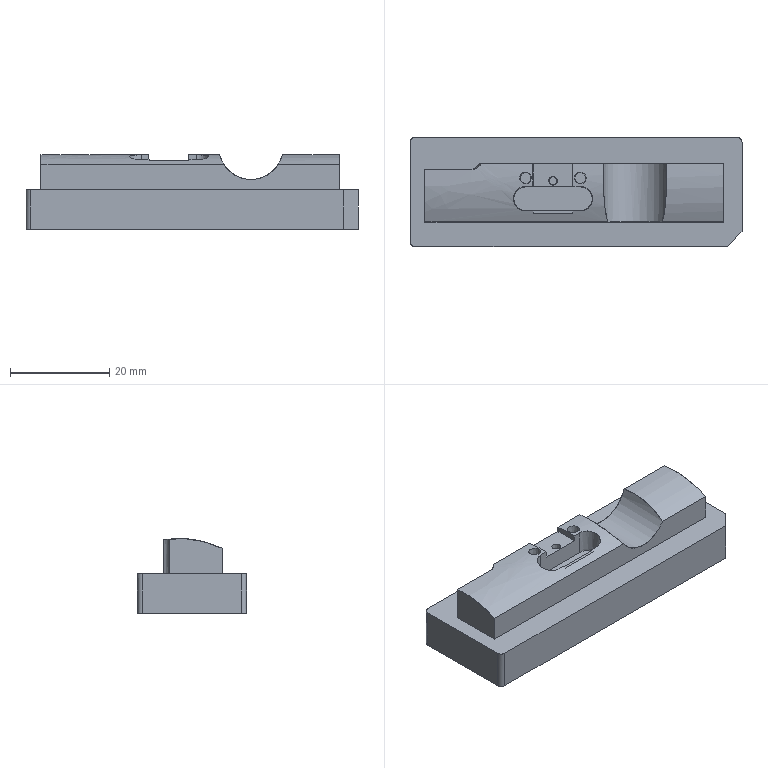NC program | PowerMill | posted with a generic post | part box 67 x 22 x 15.086 mm
Lines 3613 to 4616 of 221347:
N3710 M6
N3711 S18000 M03
N3712 G00 G90 X0.0 Y0.0
N3713 G43 Z9.7955 H15
N3714
N3715 G05 P10000 R4
N3716 X-0.6332 Y7.3349
N3717 Z0.8484
N3718 G01 Z-0.3516 F3000.0
N3719 Y7.1424 F5000.0
N3720 Y6.6108
N3721 X4.8545
N3722 X5.6988 Y6.6067
N3723 X6.1209 Y6.5128
N3724 X6.5431 Y6.2684
N3725 X6.6925 Y6.1209
N3726 X6.9624 Y5.6988
N3727 X7.0797 Y5.2767
N3728 X7.09 Y4.8545
N3729 X7.0958 Y1.0553
N3730 X7.0893 Y0.2111
N3731 X7.042 Y-0.2111
N3732 X6.9652 Y-0.4387
N3733 X6.8564 Y-0.6332
N3734 X6.4683 Y-1.0553
N3735 X6.1209 Y-1.2444
N3736 X5.6988 Y-1.3397
N3737 X2.7439 Y-1.3535
N3738 X2.3217 Y-1.2795
N3739 X1.8996 Y-1.0606
N3740 X1.4616 Y-0.6332
N3741 X1.2676 Y-0.5134
N3742 X1.0553 Y-0.4422
N3743 X1.0353 Y-0.4412
N3744 X0.6332 Y-0.42
N3745 X0.6293
N3746 X-0.6332
N3747 X-1.0553 Y-0.3626
N3748 X-1.4072 Y-0.2111
N3749 X-1.8666 Y0.2111
N3750 X-2.0765 Y0.6332
N3751 X-2.1447 Y1.0553
N3752 X-2.1446 Y4.8545
N3753 X-2.1353 Y5.2767
N3754 X-2.0179 Y5.6988
N3755 X-1.8996 Y5.9318
N3756 X-1.741 Y6.1209
N3757 X-1.4775 Y6.357
N3758 X-1.0553 Y6.5522
N3759 X-0.6332 Y6.6108
N3760 Y7.1424
N3761 G00 Z3.8484
N3762 G01 X-8.5382 Y7.3222 F10000.0
N3763 G00 Z0.8484
N3764 G01 Z-0.3516 F3000.0
N3765 X-8.569 Y7.1322 F5000.0
N3766 X-8.6537 Y6.6106
N3767 X-8.2316 Y6.542
N3768 X-7.8095 Y6.3319
N3769 X-7.5804 Y6.1209
N3770 X-7.3873 Y5.8707
N3771 X-7.3037 Y5.6988
N3772 X-7.1909 Y5.2767
N3773 X-7.1851 Y4.8545
N3774 X-7.1849 Y3.0772
N3775 X-5.3106
N3776 G02 X-4.1106 I0.6 J0.0
N3777 G02 X-5.3106 I-0.6 J0.0
N3778 G01 X-7.1849
N3779 X-7.1846 Y1.0553
N3780 X-7.2492 Y0.6332
N3781 X-7.3873 Y0.3236
N3782 X-7.4657 Y0.2111
N3783 X-7.8095 Y-0.1403
N3784 X-8.2316 Y-0.3475
N3785 X-8.6537 Y-0.4198
N3786 X-9.9201 Y-0.42
N3787 X-10.3423 Y-0.4421
N3788 X-10.557 Y-0.5125
N3789 X-10.7525 Y-0.6332
N3790 X-10.7642 Y-0.6446
N3791 X-10.7644 Y-0.6448
N3792 X-11.1848 Y-1.0553
N3793 X-11.6087 Y-1.2773
N3794 X-12.0308 Y-1.3551
N3795 X-19.6292 Y-1.3195
N3796 X-21.7399 Y-1.2703
N3797 X-29.7604 Y-1.2535
N3798 X-30.1825 Y-1.3112
N3799 X-30.6047 Y-1.3346
N3800 X-31.0268 Y-1.2356
N3801 X-31.4489 Y-0.9787
N3802 X-31.7472 Y-0.6332
N3803 X-31.8711 Y-0.3932
N3804 X-31.9294 Y-0.2111
N3805 X-31.9767 Y0.2111
N3806 Y4.4324
N3807 X-31.936 Y4.8545
N3808 X-31.8711 Y5.0606
N3809 X-31.7646 Y5.2767
N3810 X-31.4489 Y5.6498
N3811 X-31.0268 Y5.903
N3812 X-30.6047 Y6.002
N3813 X-30.1825 Y6.0075
N3814 X-21.1046 Y6.0103
N3815 X-20.8956 Y6.0394
N3816 X-20.7182 Y6.1209
N3817 X-20.4735 Y6.3206
N3818 X-20.0513 Y6.528
N3819 X-19.6292 Y6.6027
N3820 X-19.2071 Y6.6102
N3821 X-8.6537 Y6.6106
N3822 X-8.569 Y7.1322
N3823 G00 Z3.7118
N3824 G01 X6.2728 Y-2.9748 F10000.0
N3825 G00 Z0.7118
N3826 G01 Z-0.4882 F3000.0
N3827 X6.236 Y-2.7859 F5000.0
N3828 X6.1209 Y-2.1942
N3829 X5.6988 Y-2.2763
N3830 X3.166 Y-2.2705
N3831 X2.7439 Y-2.1871
N3832 X2.3217 Y-1.9541
N3833 X1.9254 Y-1.4775
N3834 X1.7658 Y-1.0553
N3835 X1.6513 Y-0.8317
N3836 X1.4881 Y-0.659
N3837 X1.4749 Y-0.6462
N3838 X1.2667 Y-0.5142
N3839 X1.0553 Y-0.4443
N3840 X0.6332 Y-0.4212
N3841 X0.6292
N3842 X-0.6332
N3843 X-1.0553 Y-0.3637
N3844 X-1.409 Y-0.2111
N3845 X-1.8675 Y0.2111
N3846 X-2.0765 Y0.6332
N3847 X-2.1447 Y1.0553
N3848 X-2.1446 Y2.2992
N3849 X-2.1445 Y4.8545
N3850 X-2.1444 Y4.8604
N3851 X-2.1443 Y5.6988
N3852 X-2.0862 Y6.1209
N3853 X-1.8996 Y6.5287
N3854 X-1.4775 Y6.9549
N3855 X-1.0553 Y7.1501
N3856 X-0.6332 Y7.2075
N3857 X5.2767
N3858 X5.6988 Y7.201
N3859 X6.1209 Y7.1257
N3860 X6.5431 Y6.8983
N3861 X6.8779 Y6.5431
N3862 X6.9652 Y6.3946
N3863 X7.074 Y6.1209
N3864 X7.1321 Y5.6988
N3865 X7.1391 Y0.2111
N3866 X7.1306 Y-0.6332
N3867 X7.0994 Y-1.0553
N3868 X6.9652 Y-1.4541
N3869 X6.6217 Y-1.8996
N3870 X6.5431 Y-1.965
N3871 X6.1209 Y-2.1942
N3872 X6.236 Y-2.7859
N3873 G00 Z3.7118
N3874 G01 X-30.7864 Y-3.0115 F10000.0
N3875 G00 Z0.7118
N3876 G01 Z-0.4882 F3000.0
N3877 X-30.7424 Y-2.8241 F5000.0
N3878 X-30.6047 Y-2.2385
N3879 X-31.0268 Y-2.1392
N3880 X-31.4489 Y-1.8933
N3881 X-31.7811 Y-1.4775
N3882 X-31.8711 Y-1.2977
N3883 X-31.9434 Y-1.0553
N3884 X-31.9767 Y-0.6332
N3885 Y4.4324
N3886 X-31.936 Y4.8545
N3887 X-31.8711 Y5.0606
N3888 X-31.7646 Y5.2767
N3889 X-31.4489 Y5.6498
N3890 X-31.0268 Y5.903
N3891 X-30.6047 Y6.002
N3892 X-30.1825 Y6.0075
N3893 X-30.0141
N3894 X-21.283 Y6.0102
N3895 X-21.2773 Y6.0106
N3896 X-20.8956 Y6.0402
N3897 X-20.7218 Y6.1209
N3898 X-20.5788 Y6.2528
N3899 X-20.3973 Y6.5431
N3900 X-20.0513 Y6.9071
N3901 X-19.6292 Y7.1274
N3902 X-19.2071 Y7.1966
N3903 X-18.7849 Y7.2075
N3904 X-8.6537 Y7.2073
N3905 X-8.2316 Y7.1271
N3906 X-7.8661 Y6.9652
N3907 X-7.4343 Y6.5431
N3908 X-7.2398 Y6.1209
N3909 X-7.184 Y5.6988
N3910 X-7.1836 Y3.7039
N3911 X-5.3179 Y3.7135
N3912 G02 X-4.7181 Y4.3166 I0.6 J0.0031
N3913 G01 X-4.6106
N3914 G02 X-4.0104 Y3.7137 I0.0002 J-0.6
N3915 G01 X-4.0136 Y3.071
N3916 G02 X-4.6144 Y2.474 I-0.6 J0.003
N3917 G01 X-4.7154 Y2.4741
N3918 G02 X-5.3146 Y3.071 I0.0008 J0.6
N3919 G01 X-5.3179 Y3.7135
N3920 X-7.1836 Y3.7039
N3921 X-7.1831 Y1.0553
N3922 X-7.2481 Y0.6332
N3923 X-7.3873 Y0.3207
N3924 X-7.4618 Y0.2111
N3925 X-7.8095 Y-0.1422
N3926 X-8.2316 Y-0.3504
N3927 X-8.6537 Y-0.421
N3928 X-9.9201 Y-0.4212
N3929 X-10.3423 Y-0.444
N3930 X-10.5561 Y-0.5133
N3931 X-10.7507 Y-0.6332
N3932 X-10.9407 Y-0.8297
N3933 X-11.0061 Y-0.9419
N3934 X-11.1865 Y-1.4214
N3935 X-11.5545 Y-1.8996
N3936 X-12.0308 Y-2.1853
N3937 X-12.4529 Y-2.2745
N3938 X-21.5288 Y-2.248
N3939 X-30.6047 Y-2.2385
N3940 X-30.7424 Y-2.8241
N3941 G00 Z3.5751
N3942 G01 X6.2495 Y-3.701 F10000.0
N3943 G00 Z0.5751
N3944 G01 Z-0.6249 F3000.0
N3945 X6.2187 Y-3.511 F5000.0
N3946 X6.1209 Y-2.9087
N3947 X5.6988 Y-2.9772
N3948 X3.166 Y-2.9741
N3949 X2.7439 Y-2.8638
N3950 X2.5152 Y-2.7439
N3951 X2.3217 Y-2.5996
N3952 X2.0811 Y-2.3217
N3953 X1.8825 Y-1.8996
N3954 X1.8231 Y-1.3709
N3955 X1.7646 Y-1.0553
N3956 X1.6505 Y-0.8325
N3957 X1.4775 Y-0.6493
N3958 X1.2659 Y-0.5151
N3959 X1.0553 Y-0.4465
N3960 X1.0363 Y-0.4454
N3961 X0.6332 Y-0.4224
N3962 X-0.6332
N3963 X-1.0553 Y-0.3647
N3964 X-1.4108 Y-0.2111
N3965 X-1.8679 Y0.2111
N3966 X-2.0765 Y0.6332
N3967 X-2.1447 Y1.0553
N3968 X-2.1445 Y3.0729
N3969 X-4.012 Y3.0724
N3970 G02 X-4.6127 Y2.4723 I-0.6 J-0.0001
N3971 G01 X-4.7153 Y2.4724
N3972 G02 X-5.3146 Y3.0725 I0.0007 J0.6
N3973 G01 X-5.3145 Y3.7085
N3974 G02 X-4.715 Y4.3083 I0.6 J-0.0002
N3975 G01 X-4.6128 Y4.3084
N3976 G02 X-4.0122 Y3.7086 I0.0006 J-0.6
N3977 G01 X-4.012 Y3.0724
N3978 X-2.1445 Y3.0729
N3979 Y3.5561
N3980 Y4.8545
N3981 X-2.1444 Y4.8575
N3982 X-2.1443 Y5.6988
N3983 X-2.0863 Y6.1209
N3984 X-1.8996 Y6.5287
N3985 X-1.4775 Y6.9549
N3986 X-1.0553 Y7.1501
N3987 X-0.6332 Y7.2075
N3988 X5.6988 Y7.2074
N3989 X6.1209 Y7.1401
N3990 X6.4963 Y6.9652
N3991 X6.9245 Y6.5431
N3992 X7.1207 Y6.1209
N3993 X7.1787 Y5.6988
N3994 X7.175 Y2.7439
N3995 X7.1818 Y-0.2111
N3996 X7.1685 Y-1.4775
N3997 X7.1065 Y-1.8996
N3998 X6.9074 Y-2.3217
N3999 X6.4747 Y-2.7439
N4000 X6.1209 Y-2.9087
N4001 X6.2187 Y-3.511
N4002 G00 Z3.5751
N4003 G01 X-31.3963 Y-3.5933 F10000.0
N4004 G00 Z0.5751
N4005 G01 Z-0.6249 F3000.0
N4006 X-31.3081 Y-3.4222 F5000.0
N4007 X-31.0268 Y-2.8762
N4008 X-31.2837 Y-2.7439
N4009 X-31.4489 Y-2.6222
N4010 X-31.7156 Y-2.3217
N4011 X-31.8711 Y-2.0325
N4012 X-31.9169 Y-1.8996
N4013 X-31.9767 Y-1.4775
N4014 Y4.4324
N4015 X-31.936 Y4.8545
N4016 X-31.8711 Y5.0606
N4017 X-31.7646 Y5.2767
N4018 X-31.4489 Y5.6498
N4019 X-31.0268 Y5.903
N4020 X-30.6047 Y6.002
N4021 X-30.1825 Y6.0075
N4022 X-29.8456
N4023 X-21.2861 Y6.0101
N4024 X-21.28 Y6.0106
N4025 X-20.8956 Y6.0427
N4026 X-20.729 Y6.1209
N4027 X-20.6745 Y6.1645
N4028 X-20.6467 Y6.1901
N4029 X-20.4045 Y6.5431
N4030 X-20.0513 Y6.9127
N4031 X-19.6292 Y7.1302
N4032 X-19.2071 Y7.199
N4033 X-18.7849 Y7.2075
N4034 X-8.6537 Y7.2073
N4035 X-8.2316 Y7.1294
N4036 X-7.8649 Y6.9652
N4037 X-7.4338 Y6.5431
N4038 X-7.2385 Y6.1209
N4039 X-7.1824 Y5.6988
N4040 X-7.1816 Y1.0553
N4041 X-7.247 Y0.6332
N4042 X-7.3873 Y0.3177
N4043 X-7.4579 Y0.2111
N4044 X-7.8095 Y-0.144
N4045 X-8.2316 Y-0.3533
N4046 X-8.6537 Y-0.4222
N4047 X-9.9201 Y-0.4224
N4048 X-10.3423 Y-0.446
N4049 X-10.5552 Y-0.5142
N4050 X-10.7488 Y-0.6332
N4051 X-10.9398 Y-0.8306
N4052 X-11.0288 Y-1.0022
N4053 X-11.0678 Y-1.1057
N4054 X-11.1035 Y-1.2636
N4055 X-11.1725 Y-1.8996
N4056 X-11.3736 Y-2.3217
N4057 X-11.6087 Y-2.5959
N4058 X-11.8055 Y-2.7439
N4059 X-12.0308 Y-2.8613
N4060 X-12.4529 Y-2.969
N4061 X-12.8751 Y-2.9803
N4062 X-26.3833 Y-2.9814
N4063 X-30.6047 Y-2.9752
N4064 X-31.0268 Y-2.8762
N4065 X-31.3081 Y-3.4222
N4066 G00 Z3.4385
N4067 G01 X3.4817 Y-4.3843 F10000.0
N4068 G00 Z0.4385
N4069 G01 Z-0.7615 F3000.0
N4070 X3.4819 Y-4.1918 F5000.0
N4071 X3.4826 Y-3.5739
N4072 X3.166 Y-3.5736
N4073 X2.7439 Y-3.4944
N4074 X2.3217 Y-3.2749
N4075 X2.1907 Y-3.166
N4076 X1.8996 Y-2.7873
N4077 X1.7385 Y-2.3217
N4078 X1.7269 Y-1.8996
N4079 X1.8143 Y-1.4775
N4080 X1.812 Y-1.3107
N4081 X1.77 Y-1.0845
N4082 X1.7633 Y-1.0553
N4083 X1.6496 Y-0.8334
N4084 X1.4775 Y-0.6509
N4085 X1.4619 Y-0.641
N4086 X1.2657 Y-0.5164
N4087 X1.0553 Y-0.4483
N4088 X0.6332 Y-0.4236
N4089 X-0.6332
N4090 X-1.0553 Y-0.3658
N4091 X-1.4125 Y-0.2111
N4092 X-1.8682 Y0.2111
N4093 X-2.0765 Y0.6332
N4094 X-2.1447 Y1.0553
N4095 X-2.1444 Y4.8546
N4096 X-2.1443 Y5.6988
N4097 X-2.0863 Y6.1209
N4098 X-1.8996 Y6.5287
N4099 X-1.4775 Y6.9549
N4100 X-1.0553 Y7.1502
N4101 X-0.6332 Y7.2075
N4102 X5.6988
N4103 X6.1209 Y7.1544
N4104 X6.5431 Y6.9646
N4105 X6.9652 Y6.5515
N4106 X7.1673 Y6.1209
N4107 X7.2254 Y5.6988
N4108 X7.2183 Y-1.8996
N4109 X7.1904 Y-2.3217
N4110 X7.0509 Y-2.7439
N4111 X6.9652 Y-2.899
N4112 X6.7402 Y-3.166
N4113 X6.5431 Y-3.3229
N4114 X6.1209 Y-3.5176
N4115 X5.6988 Y-3.5765
N4116 X3.4826 Y-3.5739
N4117 X3.4819 Y-4.1918
N4118 G00 Z3.4385
N4119 G01 X-30.7863 Y-4.3518 F10000.0
N4120 G00 Z0.4385
N4121 G01 Z-0.7615 F3000.0
N4122 X-30.7434 Y-4.1641 F5000.0
N4123 X-30.6047 Y-3.5569
N4124 X-31.0268 Y-3.4605
N4125 X-31.4489 Y-3.2042
N4126 X-31.8112 Y-2.7439
N4127 X-31.8711 Y-2.6162
N4128 X-31.953 Y-2.3217
N4129 X-31.9767 Y-1.8996
N4130 Y4.4324
N4131 X-31.936 Y4.8545
N4132 X-31.8711 Y5.0606
N4133 X-31.7646 Y5.2767
N4134 X-31.4489 Y5.6498
N4135 X-31.0268 Y5.903
N4136 X-30.6047 Y6.002
N4137 X-30.1825 Y6.0075
N4138 X-29.677
N4139 X-21.2888 Y6.0101
N4140 X-21.2823 Y6.0107
N4141 X-20.8956 Y6.0452
N4142 X-20.7362 Y6.1209
N4143 X-20.6568 Y6.1849
N4144 X-20.4116 Y6.5431
N4145 X-20.0513 Y6.9177
N4146 X-19.6292 Y7.133
N4147 X-19.2071 Y7.2013
N4148 X-18.7849 Y7.2075
N4149 X-8.6537 Y7.2073
N4150 X-8.2316 Y7.1317
N4151 X-7.8637 Y6.9652
N4152 X-7.4332 Y6.5431
N4153 X-7.2372 Y6.1209
N4154 X-7.1808 Y5.6988
N4155 X-7.1805 Y3.7046
N4156 X-5.3179 Y3.7141
N4157 G02 X-4.7176 Y4.3171 I0.6 J0.003
N4158 G01 X-4.6069
N4159 G02 X-4.0073 Y3.7141 I-0.0003 J-0.6
N4160 G01 X-4.0105 Y3.0676
N4161 G02 X-4.611 Y2.4706 I-0.6 J0.003
N4162 G01 X-4.7152 Y2.4707
N4163 G02 X-5.3146 Y3.0676 I0.0005 J0.6
N4164 G01 X-5.3179 Y3.7141
N4165 X-7.1805 Y3.7046
N4166 X-7.1801 Y1.0553
N4167 X-7.246 Y0.6332
N4168 X-7.2569 Y0.6109
N4169 X-7.3874 Y0.3177
N4170 X-7.4424 Y0.2346
N4171 X-7.454 Y0.2111
N4172 X-7.8095 Y-0.1458
N4173 X-8.2316 Y-0.356
N4174 X-8.6537 Y-0.4234
N4175 X-9.9201 Y-0.4236
N4176 X-10.3423 Y-0.4479
N4177 X-10.5543 Y-0.5151
N4178 X-10.7469 Y-0.6332
N4179 X-10.939 Y-0.8314
N4180 X-11.0329 Y-1.0128
N4181 X-11.0641 Y-1.0958
N4182 X-11.1023 Y-1.2636
N4183 X-11.1055 Y-1.4775
N4184 X-11.0168 Y-1.8996
N4185 X-11.03 Y-2.3217
N4186 X-11.1694 Y-2.7439
N4187 X-11.484 Y-3.166
N4188 X-11.6087 Y-3.2735
N4189 X-12.0308 Y-3.4966
N4190 X-12.4529 Y-3.5753
N4191 X-30.1825 Y-3.5447
N4192 X-30.6047 Y-3.5569
N4193 X-30.7434 Y-4.1641
N4194 G00 Z3.3019
N4195 G01 X2.0512 Y-4.7063 F10000.0
N4196 G00 Z0.3019
N4197 G01 Z-0.8981 F3000.0
N4198 X2.1256 Y-4.5288 F5000.0
N4199 X2.3665 Y-3.954
N4200 X2.3217 Y-3.9353
N4201 X1.8996 Y-3.6208
N4202 X1.6087 Y-3.166
N4203 X1.5028 Y-2.7439
N4204 X1.5234 Y-2.3217
N4205 X1.7223 Y-1.801
N4206 X1.8121 Y-1.4775
N4207 X1.8105 Y-1.3024
N4208 X1.7754 Y-1.1133
N4209 X1.7747 Y-1.1102
N4210 X1.7621 Y-1.0553
N4211 X1.6488 Y-0.8343
N4212 X1.4775 Y-0.6524
N4213 X1.2647 Y-0.5172
N4214 X1.0553 Y-0.4495
N4215 X0.6332 Y-0.4248
N4216 X-0.6332
N4217 X-1.0553 Y-0.3668
N4218 X-1.4141 Y-0.2111
N4219 X-1.8685 Y0.2111
N4220 X-2.0765 Y0.6332
N4221 X-2.1447 Y1.0553
N4222 X-2.1446 Y3.0692
N4223 X-4.0089 Y3.0689
N4224 G02 X-4.6094 Y2.4688 I-0.6 J-0.0001
N4225 G01 X-4.7151 Y2.4689
N4226 G02 X-5.3147 Y3.069 I0.0004 J0.6
N4227 G01 X-5.3145 Y3.709
N4228 G02 X-4.7147 Y4.3089 I0.6 J-0.0001
N4229 G01 X-4.6092
N4230 G02 X-4.009 Y3.709 I0.0002 J-0.6
N4231 G01 X-4.0089 Y3.0689
N4232 X-2.1446 Y3.0692
N4233 X-2.1443 Y5.6988
N4234 X-2.0863 Y6.1209
N4235 X-1.8996 Y6.5287
N4236 X-1.4775 Y6.9549
N4237 X-1.0553 Y7.1502
N4238 X-0.6332 Y7.2075
N4239 X5.6988
N4240 X6.1209 Y7.1663
N4241 X6.5431 Y6.9934
N4242 X6.9652 Y6.6161
N4243 X7.2139 Y6.1209
N4244 X7.272 Y5.6988
N4245 X7.2644 Y5.2767
N4246 X7.2658 Y-2.3217
N4247 X7.2506 Y-2.7439
N4248 X7.1436 Y-3.166
N4249 X6.8832 Y-3.5881
N4250 X6.5431 Y-3.8709
N4251 X6.2509 Y-4.0103
N4252 X6.1209 Y-4.0532
N4253 X5.6988 Y-4.0979
N4254 X3.166 Y-4.0987
N4255 X2.7439 Y-4.0735
N4256 X2.5007 Y-4.0103
N4257 X2.3665 Y-3.954
N4258 X2.1256 Y-4.5288
N4259 G00 Z3.3019
N4260 G01 X-11.5869 Y-4.7929 F10000.0
N4261 G00 Z0.3019
N4262 G01 Z-0.8981 F3000.0
N4263 X-11.6356 Y-4.6066 F5000.0
N4264 X-11.7914 Y-4.0103
N4265 X-12.0308 Y-4.0728
N4266 X-12.4529 Y-4.0989
N4267 X-25.1169 Y-4.0572
N4268 X-30.6047 Y-4.0625
N4269 X-31.0268 Y-3.9629
N4270 X-31.4489 Y-3.7097
N4271 X-31.5726 Y-3.5881
N4272 X-31.8503 Y-3.166
N4273 X-31.9655 Y-2.7439
N4274 X-31.9767 Y-2.3217
N4275 Y4.4324
N4276 X-31.936 Y4.8545
N4277 X-31.8711 Y5.0606
N4278 X-31.7646 Y5.2767
N4279 X-31.4489 Y5.6498
N4280 X-31.0268 Y5.903
N4281 X-30.6047 Y6.002
N4282 X-30.0565 Y6.0083
N4283 X-29.5082 Y6.0075
N4284 X-21.2912 Y6.01
N4285 X-21.2843 Y6.0107
N4286 X-20.8956 Y6.0477
N4287 X-20.7434 Y6.1209
N4288 X-20.6617 Y6.1871
N4289 X-20.4188 Y6.5431
N4290 X-20.0513 Y6.9228
N4291 X-19.6292 Y7.1358
N4292 X-19.2071 Y7.2037
N4293 X-18.7849 Y7.2075
N4294 X-8.6537 Y7.2073
N4295 X-8.2316 Y7.1341
N4296 X-7.8625 Y6.9652
N4297 X-7.4327 Y6.5431
N4298 X-7.2365 Y6.1209
N4299 X-7.1793 Y5.6988
N4300 X-7.1786 Y1.0553
N4301 X-7.2451 Y0.6332
N4302 X-7.2665 Y0.5895
N4303 X-7.3874 Y0.3177
N4304 X-7.4362 Y0.2441
N4305 X-7.4524 Y0.2111
N4306 X-7.8095 Y-0.1474
N4307 X-8.2316 Y-0.3586
N4308 X-8.6537 Y-0.4246
N4309 X-9.9201 Y-0.4248
N4310 X-10.3423 Y-0.4491
N4311 X-10.554 Y-0.5163
N4312 X-10.7451 Y-0.6332
N4313 X-10.9381 Y-0.8322
N4314 X-11.037 Y-1.0235
N4315 X-11.0603 Y-1.0856
N4316 X-11.1011 Y-1.2637
N4317 X-11.1027 Y-1.4775
N4318 X-11.0523 Y-1.6945
N4319 X-10.8153 Y-2.3217
N4320 X-10.7946 Y-2.7439
N4321 X-10.9016 Y-3.166
N4322 X-11.1662 Y-3.5881
N4323 X-11.6087 Y-3.9318
N4324 X-11.7914 Y-4.0103
N4325 X-11.6356 Y-4.6066
N4326 G00 Z3.1653
N4327 G01 X0.7672 Y-4.4152 F10000.0
N4328 G00 Z0.1653
N4329 G01 Z-1.0347 F3000.0
N4330 X0.9348 Y-4.3206 F5000.0
N4331 X1.4775 Y-4.0145
N4332 X1.2369 Y-3.5881
N4333 X1.1457 Y-3.166
N4334 X1.1778 Y-2.7439
N4335 X1.3409 Y-2.3217
N4336 X1.7188 Y-1.8038
N4337 X1.81 Y-1.4775
N4338 X1.8091 Y-1.2944
N4339 X1.7807 Y-1.1416
N4340 X1.78 Y-1.1384
N4341 X1.7608 Y-1.0553
N4342 X1.648 Y-0.8352
N4343 X1.4775 Y-0.6539
N4344 X1.2637 Y-0.518
N4345 X1.0553 Y-0.4507
N4346 X0.6332 Y-0.426
N4347 X-0.6332
N4348 X-1.0553 Y-0.3679
N4349 X-1.4156 Y-0.2111
N4350 X-1.8688 Y0.2111
N4351 X-2.0765 Y0.6332
N4352 X-2.1447 Y1.0553
N4353 X-2.1444 Y5.6988
N4354 X-2.0863 Y6.1209
N4355 X-1.8996 Y6.5287
N4356 X-1.4775 Y6.9549
N4357 X-1.0553 Y7.1502
N4358 X-0.6332 Y7.2075
N4359 X5.6988
N4360 X6.1209 Y7.1763
N4361 X6.5431 Y7.0207
N4362 X6.6362 Y6.9652
N4363 X6.9652 Y6.6745
N4364 X7.0644 Y6.5431
N4365 X7.2606 Y6.1209
N4366 X7.3186 Y5.6988
N4367 X7.309 Y5.2767
N4368 X7.3099 Y-2.7439
N4369 X7.3051 Y-3.166
N4370 X7.2132 Y-3.5881
N4371 X6.9652 Y-4.0212
N4372 X6.5431 Y-4.3731
N4373 X6.4244 Y-4.4324
N4374 X6.1209 Y-4.5332
N4375 X5.6988 Y-4.566
N4376 X2.7439 Y-4.5657
N4377 X2.3217 Y-4.5328
N4378 X2.0184 Y-4.4324
N4379 X1.8996 Y-4.3691
N4380 X1.4775 Y-4.0145
N4381 X0.9348 Y-4.3206
N4382 G00 Z3.1653
N4383 G01 X-10.8258 Y-5.1025 F10000.0
N4384 G00 Z0.1653
N4385 G01 Z-1.0347 F3000.0
N4386 X-10.9106 Y-4.9297 F5000.0
N4387 X-11.1865 Y-4.3677
N4388 X-11.3183 Y-4.4324
N4389 X-11.6087 Y-4.5281
N4390 X-12.0308 Y-4.567
N4391 X-30.6047 Y-4.5461
N4392 X-31.0503 Y-4.4324
N4393 X-31.4489 Y-4.1939
N4394 X-31.6289 Y-4.0103
N4395 X-31.8711 Y-3.6049
N4396 X-31.9707 Y-3.166
N4397 X-31.9767 Y-2.7439
N4398 Y4.4324
N4399 X-31.936 Y4.8545
N4400 X-31.8711 Y5.0606
N4401 X-31.7646 Y5.2767
N4402 X-31.4489 Y5.6498
N4403 X-31.0268 Y5.903
N4404 X-30.6047 Y6.002
N4405 X-29.972 Y6.0088
N4406 X-29.3393 Y6.0075
N4407 X-21.2933 Y6.01
N4408 X-20.9294 Y6.0469
N4409 X-20.8968 Y6.0539
N4410 X-20.8666 Y6.0679
N4411 X-20.6945 Y6.1725
N4412 X-20.6691 Y6.1919
N4413 X-20.6484 Y6.2163
N4414 X-20.426 Y6.5431
N4415 X-20.0513 Y6.9278
N4416 X-19.6292 Y7.1386
N4417 X-19.2071 Y7.206
N4418 X-18.9372 Y7.2061
N4419 X-18.9366
N4420 X-18.7849 Y7.2074
N4421 X-9.1043 Y7.2073
N4422 X-8.6537
N4423 X-8.2316 Y7.1364
N4424 X-7.8613 Y6.9652
N4425 X-7.4322 Y6.5431
N4426 X-7.236 Y6.1209
N4427 X-7.1779 Y5.6988
N4428 X-7.178 Y3.7053
N4429 X-5.318 Y3.7146
N4430 G02 X-4.7174 Y4.3176 I0.6 J0.003
N4431 G01 X-4.604 Y4.3175
N4432 G02 X-4.0046 Y3.7143 I-0.0006 J-0.6
N4433 G01 X-4.008 Y3.0639
N4434 G02 X-4.6086 Y2.4671 I-0.6 J0.0032
N4435 G01 X-4.7153 Y2.4672
N4436 G02 X-5.3147 Y3.0642 I0.0006 J0.6
N4437 G01 X-5.318 Y3.7146
N4438 X-7.178 Y3.7053
N4439 Y1.0553
N4440 X-7.2442 Y0.6332
N4441 X-7.2765 Y0.5672
N4442 X-7.3875 Y0.3178
N4443 X-7.4227 Y0.2665
N4444 X-7.451 Y0.2111
N4445 X-7.8095 Y-0.149
N4446 X-8.2316 Y-0.3612
N4447 X-8.6537 Y-0.4258
N4448 X-9.9201 Y-0.426
N4449 X-10.3423 Y-0.4503
N4450 X-10.553 Y-0.5171
N4451 X-10.7432 Y-0.6332
N4452 X-10.9373 Y-0.8331
N4453 X-11.0411 Y-1.0345
N4454 X-11.0565 Y-1.0753
N4455 X-11.0999 Y-1.2638
N4456 X-11.1006 Y-1.4775
N4457 X-11.0091 Y-1.8026
N4458 X-10.6321 Y-2.3217
N4459 X-10.4687 Y-2.7439
N4460 X-10.4359 Y-3.166
N4461 X-10.5271 Y-3.5881
N4462 X-10.7703 Y-4.0103
N4463 X-11.1865 Y-4.3677
N4464 X-10.9106 Y-4.9297
N4465 G00 Z3.0286
N4466 G01 X0.4445 Y-5.1446 F10000.0
N4467 G00 Z0.0286
N4468 G01 Z-1.1714 F3000.0
N4469 X0.5881 Y-5.0164 F5000.0
N4470 X1.0553 Y-4.5993
N4471 X0.9063 Y-4.4324
N4472 X0.6665 Y-4.0103
N4473 X0.579 Y-3.5881
N4474 X0.6109 Y-3.166
N4475 X0.7779 Y-2.7439
N4476 X1.0553 Y-2.399
N4477 X1.4775 Y-2.1048
N4478 X1.5957 Y-1.973
N4479 X1.6999 Y-1.8299
N4480 X1.7134 Y-1.8074
N4481 X1.7227 Y-1.7829
N4482 X1.8084 Y-1.4775
N4483 X1.8078 Y-1.2875
N4484 X1.7861 Y-1.1701
N4485 X1.7595 Y-1.0553
N4486 X1.6472 Y-0.8361
N4487 X1.4775 Y-0.6555
N4488 X1.2627 Y-0.5188
N4489 X1.0553 Y-0.4519
N4490 X0.6332 Y-0.4272
N4491 X-0.6332
N4492 X-1.0553 Y-0.3689
N4493 X-1.417 Y-0.2111
N4494 X-1.8691 Y0.2111
N4495 X-2.0766 Y0.6332
N4496 X-2.1448 Y1.0553
N4497 X-2.1444 Y5.6988
N4498 X-2.0863 Y6.1209
N4499 X-1.8996 Y6.5287
N4500 X-1.4775 Y6.9549
N4501 X-1.0553 Y7.1502
N4502 X-0.6332 Y7.2075
N4503 X5.6988
N4504 X6.1209 Y7.1859
N4505 X6.5431 Y7.0476
N4506 X6.6875 Y6.9652
N4507 X6.9652 Y6.7312
N4508 X7.1152 Y6.5431
N4509 X7.3114 Y6.1209
N4510 X7.3694 Y5.6988
N4511 X7.3716 Y-3.166
N4512 X7.3641 Y-3.5881
N4513 X7.2722 Y-4.0103
N4514 X7.0347 Y-4.4324
N4515 X6.9652 Y-4.5127
N4516 X6.4925 Y-4.8545
N4517 X6.1209 Y-4.973
N4518 X5.6988 Y-4.9956
N4519 X2.3217 Y-4.9968
N4520 X1.8996 Y-4.985
N4521 X1.4775 Y-4.8741
N4522 X1.0553 Y-4.5993
N4523 X0.5881 Y-5.0164
N4524 G00 Z3.0286
N4525 G01 X-9.6238 Y-4.9977 F10000.0
N4526 G00 Z0.0286
N4527 G01 Z-1.1714 F3000.0
N4528 X-9.7614 Y-4.863 F5000.0
N4529 X-10.201 Y-4.4324
N4530 X-10.3423 Y-4.5766
N4531 X-10.7513 Y-4.8545
N4532 X-11.1865 Y-4.9829
N4533 X-15.83 Y-4.9911
N4534 X-30.1825 Y-4.9767
N4535 X-30.6047 Y-4.9841
N4536 X-31.0268 Y-4.8851
N4537 X-31.4489 Y-4.632
N4538 X-31.64 Y-4.4324
N4539 X-31.8711 Y-4.0427
N4540 X-31.972 Y-3.5881
N4541 X-31.9767 Y-3.166
N4542 Y4.4324
N4543 X-31.936 Y4.8545
N4544 X-31.8711 Y5.0606
N4545 X-31.7646 Y5.2767
N4546 X-31.4489 Y5.6498
N4547 X-31.0268 Y5.903
N4548 X-30.6047 Y6.002
N4549 X-29.8882 Y6.0094
N4550 X-29.1716 Y6.0075
N4551 X-21.2933 Y6.0099
N4552 X-20.9343 Y6.0463
N4553 X-20.9018 Y6.0534
N4554 X-20.8717 Y6.0676
N4555 X-20.6988 Y6.1748
N4556 X-20.674 Y6.1941
N4557 X-20.6537 Y6.2181
N4558 X-20.4332 Y6.5431
N4559 X-20.0513 Y6.9328
N4560 X-19.6292 Y7.141
N4561 X-19.2071 Y7.2074
N4562 X-8.6537
N4563 X-8.2316 Y7.1387
N4564 X-7.8601 Y6.9652
N4565 X-7.4316 Y6.5431
N4566 X-7.2355 Y6.1209
N4567 X-7.1774 Y5.6988
N4568 Y3.706
N4569 X-5.318 Y3.7151
N4570 G02 X-4.7168 Y4.318 I0.6 J0.0029
N4571 G01 X-4.6028 Y4.3177
N4572 G02 X-4.0041 Y3.7147 I-0.0013 J-0.6
N4573 G01 X-4.0076 Y3.021
N4574 G02 X-4.6081 Y2.424 I-0.5999 J0.003
N4575 G01 X-4.7152 Y2.4241
N4576 G02 X-5.3146 Y3.0212 I0.0006 J0.6
N4577 G01 X-5.318 Y3.7151
N4578 X-7.1774 Y3.706
N4579 X-7.1775 Y1.0553
N4580 X-7.2433 Y0.6332
N4581 X-7.3411 Y0.4195
N4582 X-7.4496 Y0.2111
N4583 X-7.8095 Y-0.1506
N4584 X-8.2316 Y-0.3637
N4585 X-8.6537 Y-0.427
N4586 X-9.9201 Y-0.4272
N4587 X-10.3423 Y-0.4515
N4588 X-10.5519 Y-0.5179
N4589 X-10.7413 Y-0.6332
N4590 X-10.9367 Y-0.8342
N4591 X-11.045 Y-1.0446
N4592 X-11.0529 Y-1.0656
N4593 X-11.0988 Y-1.2641
N4594 X-11.0994 Y-1.4775
N4595 X-11.094 Y-1.5011
N4596 X-11.024 Y-1.7497
N4597 X-10.9798 Y-1.843
N4598 X-10.8905 Y-1.9659
N4599 X-10.7644 Y-2.0999
N4600 X-10.3423 Y-2.4143
N4601 X-10.0829 Y-2.7439
N4602 X-9.9116 Y-3.166
N4603 X-9.8808 Y-3.5881
N4604 X-9.9641 Y-4.0103
N4605 X-10.201 Y-4.4324
N4606 X-9.7614 Y-4.863
N4607 G00 Z2.892
N4608 G01 X7.6725 Y-5.4194 F10000.0
N4609 G00 Z-0.108
N4610 G01 Z-1.308 F3000.0
N4611 X7.5322 Y-5.2876 F5000.0
N4612 X7.0712 Y-4.8545
N4613 X6.9652 Y-4.9673
N4614 X6.4964 Y-5.2767
N4615 X6.1209 Y-5.3787
N4616 X-0.6332 Y-5.394
N4617 X-1.0553 Y-5.3356
N4618 X-1.4775 Y-5.139
N4619 X-1.7906 Y-4.8545
N4620 X-1.8996 Y-4.7098
N4621 X-2.0393 Y-4.4324
N4622 X-2.1361 Y-4.0103
N4623 X-2.1229 Y-3.5881
N4624 X-1.9911 Y-3.166
N4625 X-1.8996 Y-3.012
N4626 X-1.6862 Y-2.7439
N4627 X-1.4775 Y-2.582
N4628 X-1.0553 Y-2.3854
N4629 X-0.7273 Y-2.3217
N4630 X1.0553 Y-2.3019
N4631 X1.1667 Y-2.2691
N4632 X1.4775 Y-2.1032
N4633 X1.5979 Y-1.9694
N4634 X1.7033 Y-1.8236
N4635 X1.7147 Y-1.8035
N4636 X1.8072 Y-1.4775
N4637 X1.8066 Y-1.2807
N4638 X1.7913 Y-1.1978
N4639 X1.7583 Y-1.0553
N4640 X1.6465 Y-0.8371
N4641 X1.4775 Y-0.657
N4642 X1.2617 Y-0.5196
N4643 X1.0553 Y-0.4531
N4644 X0.6332 Y-0.4284
N4645 X-0.6332
N4646 X-1.0553 Y-0.3736
N4647 X-1.4184 Y-0.2111
N4648 X-1.8694 Y0.2111
N4649 X-2.0766 Y0.6332
N4650 X-2.1448 Y1.0553
N4651 X-2.1445 Y3.7714
N4652 X-4.0082 Y3.7243
N4653 X-4.0097 Y3.6646
N4654 X-4.0171 Y3.6053
N4655 X-4.0551 Y3.3888
N4656 G03 X-3.7495 Y-0.1667 I6.8444 J-1.2026
N4657 G01 X-3.3835 Y-1.1838
N4658 G02 X-3.4747 Y-1.7556 I-0.5646 J-0.2032
N4659 G01 X-3.7938 Y-2.1653
N4660 G02 X-4.2665 Y-2.3967 I-0.4733 J0.3686
N4661 G01 X-5.0467 Y-2.3976
N4662 G02 X-5.5285 Y-2.1561 I-0.0007 J0.6
N4663 G01 X-5.8481 Y-1.7274
N4664 G02 X-5.9291 Y-1.159 I0.4811 J0.3586
N4665 G01 X-5.4677 Y0.0771
N4666 G03 X-5.2536 Y3.3781 I-5.3736 J2.0059
N4667 G01 X-5.2991 Y3.5743
N4668 G02 X-4.7111 Y4.3097 I0.5845 J0.1354
N4669 G01 X-4.6045 Y4.3091
N4670 G02 X-4.0082 Y3.7243 I-0.0035 J-0.6
N4671 G01 X-2.1445 Y3.7714
N4672 X-2.1444 Y5.6988
N4673 X-2.0863 Y6.1209
N4674 X-1.8996 Y6.5287
N4675 X-1.4775 Y6.9549
N4676 X-1.0553 Y7.1502
N4677 X-0.6332 Y7.2075
N4678 X5.6988
N4679 X6.1209 Y7.1952
N4680 X6.5431 Y7.0762
N4681 X6.7484 Y6.9652
N4682 X6.9652 Y6.793
N4683 X7.1761 Y6.5431
N4684 X7.3727 Y6.1209
N4685 X7.4304 Y5.6988
N4686 X7.422 Y-4.0103
N4687 X7.3203 Y-4.4324
N4688 X7.0712 Y-4.8545
N4689 X7.5322 Y-5.2876
N4690 G00 Z2.892
N4691 G01 X-32.0384 Y-5.593 F10000.0
N4692 G00 Z-0.108
N4693 G01 Z-1.308 F3000.0
N4694 X-31.9014 Y-5.4578 F5000.0
N4695 X-31.4489 Y-5.0111
N4696 X-31.6035 Y-4.8545
N4697 X-31.8665 Y-4.4324
N4698 X-31.9685 Y-4.0103
N4699 X-31.9767 Y-3.5881
N4700 Y4.4324
N4701 X-31.936 Y4.8545
N4702 X-31.8711 Y5.0606
N4703 X-31.7646 Y5.2767
N4704 X-31.4489 Y5.6498
N4705 X-31.0268 Y5.903
N4706 X-30.6047 Y6.002
N4707 X-29.8036 Y6.0099
N4708 X-29.0025 Y6.0075
N4709 X-21.2933 Y6.0099
N4710 X-20.9547 Y6.0442
N4711 X-20.9165 Y6.0514
N4712 X-20.8905 Y6.0588
N4713 X-20.8663 Y6.0709